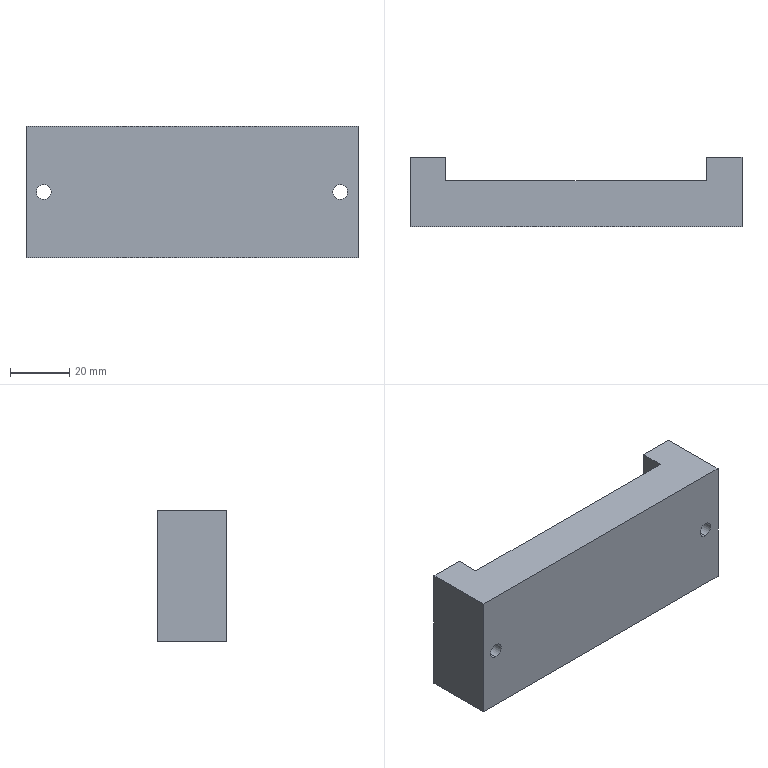Part | SolidWorks | features BaseBody 1 | 1 solid | 14 faces | box 112 x 23.5 x 44.5 mm | volume 84873 mm3 | plane 10 | cylinder 4 | commonest cylinder face diameters 5 x4
STEP:
#1=CARTESIAN_POINT('',(50.,-108.5,226.731));
#2=VERTEX_POINT('',#1);
#3=CARTESIAN_POINT('',(50.,-108.5,221.731));
#4=VERTEX_POINT('',#3);
#5=CARTESIAN_POINT('',(50.,-108.5,224.231));
#6=DIRECTION('',(0.,-1.,0.));
#7=DIRECTION('',(0.,0.,1.));
#8=AXIS2_PLACEMENT_3D('',#5,#6,#7);
#9=CIRCLE('',#8,2.5);
#10=EDGE_CURVE('',#2,#4,#9,.T.);
#11=ORIENTED_EDGE('',*,*,#10,.T.);
#12=CARTESIAN_POINT('',(50.,-85.,221.731));
#13=VERTEX_POINT('',#12);
#14=CARTESIAN_POINT('',(50.,-85.,221.731));
#15=DIRECTION('',(0.,1.,0.));
#16=VECTOR('',#15,1000.);
#17=LINE('',#14,#16);
#18=EDGE_CURVE('',#4,#13,#17,.T.);
#19=ORIENTED_EDGE('',*,*,#18,.T.);
#20=CARTESIAN_POINT('',(50.,-85.,226.731));
#21=VERTEX_POINT('',#20);
#22=CARTESIAN_POINT('',(50.,-85.,224.231));
#23=DIRECTION('',(0.,-1.,0.));
#24=DIRECTION('',(0.,0.,1.));
#25=AXIS2_PLACEMENT_3D('',#22,#23,#24);
#26=CIRCLE('',#25,2.5);
#27=EDGE_CURVE('',#21,#13,#26,.T.);
#28=ORIENTED_EDGE('',*,*,#27,.F.);
#29=CARTESIAN_POINT('',(50.,-85.,226.731));
#30=DIRECTION('',(0.,1.,0.));
#31=VECTOR('',#30,1000.);
#32=LINE('',#29,#31);
#33=EDGE_CURVE('',#2,#21,#32,.T.);
#34=ORIENTED_EDGE('',*,*,#33,.F.);
#35=EDGE_LOOP('',(#11,#19,#28,#34));
#36=FACE_OUTER_BOUND('',#35,.T.);
#37=CARTESIAN_POINT('',(50.,-85.,224.231));
#38=DIRECTION('',(0.,1.,0.));
#39=DIRECTION('',(0.,0.,1.));
#40=AXIS2_PLACEMENT_3D('',#37,#38,#39);
#41=CYLINDRICAL_SURFACE('',#40,2.5);
#42=ADVANCED_FACE('',(#36),#41,.F.);
#43=CARTESIAN_POINT('',(-50.,-108.5,226.731));
#44=VERTEX_POINT('',#43);
#45=CARTESIAN_POINT('',(-50.,-108.5,221.731));
#46=VERTEX_POINT('',#45);
#47=CARTESIAN_POINT('',(-50.,-108.5,224.231));
#48=DIRECTION('',(0.,-1.,0.));
#49=DIRECTION('',(0.,0.,1.));
#50=AXIS2_PLACEMENT_3D('',#47,#48,#49);
#51=CIRCLE('',#50,2.5);
#52=EDGE_CURVE('',#44,#46,#51,.T.);
#53=ORIENTED_EDGE('',*,*,#52,.T.);
#54=CARTESIAN_POINT('',(-50.,-85.,221.731));
#55=VERTEX_POINT('',#54);
#56=CARTESIAN_POINT('',(-50.,-85.,221.731));
#57=DIRECTION('',(0.,1.,0.));
#58=VECTOR('',#57,1000.);
#59=LINE('',#56,#58);
#60=EDGE_CURVE('',#46,#55,#59,.T.);
#61=ORIENTED_EDGE('',*,*,#60,.T.);
#62=CARTESIAN_POINT('',(-50.,-85.,226.731));
#63=VERTEX_POINT('',#62);
#64=CARTESIAN_POINT('',(-50.,-85.,224.231));
#65=DIRECTION('',(0.,-1.,0.));
#66=DIRECTION('',(0.,0.,1.));
#67=AXIS2_PLACEMENT_3D('',#64,#65,#66);
#68=CIRCLE('',#67,2.5);
#69=EDGE_CURVE('',#63,#55,#68,.T.);
#70=ORIENTED_EDGE('',*,*,#69,.F.);
#71=CARTESIAN_POINT('',(-50.,-85.,226.731));
#72=DIRECTION('',(0.,1.,0.));
#73=VECTOR('',#72,1000.);
#74=LINE('',#71,#73);
#75=EDGE_CURVE('',#44,#63,#74,.T.);
#76=ORIENTED_EDGE('',*,*,#75,.F.);
#77=EDGE_LOOP('',(#53,#61,#70,#76));
#78=FACE_OUTER_BOUND('',#77,.T.);
#79=CARTESIAN_POINT('',(-50.,-85.,224.231));
#80=DIRECTION('',(0.,1.,0.));
#81=DIRECTION('',(0.,0.,1.));
#82=AXIS2_PLACEMENT_3D('',#79,#80,#81);
#83=CYLINDRICAL_SURFACE('',#82,2.5);
#84=ADVANCED_FACE('',(#78),#83,.F.);
#85=CARTESIAN_POINT('',(56.,-108.5,246.481));
#86=VERTEX_POINT('',#85);
#87=CARTESIAN_POINT('',(56.,-108.5,201.981));
#88=VERTEX_POINT('',#87);
#89=CARTESIAN_POINT('',(56.,-108.5,246.481));
#90=DIRECTION('',(0.,0.,-1.));
#91=VECTOR('',#90,1000.);
#92=LINE('',#89,#91);
#93=EDGE_CURVE('',#86,#88,#92,.T.);
#94=ORIENTED_EDGE('',*,*,#93,.F.);
#95=CARTESIAN_POINT('',(-56.,-108.5,246.481));
#96=VERTEX_POINT('',#95);
#97=CARTESIAN_POINT('',(-56.,-108.5,246.481));
#98=DIRECTION('',(1.,0.,0.));
#99=VECTOR('',#98,1000.);
#100=LINE('',#97,#99);
#101=EDGE_CURVE('',#96,#86,#100,.T.);
#102=ORIENTED_EDGE('',*,*,#101,.F.);
#103=CARTESIAN_POINT('',(-56.,-108.5,201.981));
#104=VERTEX_POINT('',#103);
#105=CARTESIAN_POINT('',(-56.,-108.5,246.481));
#106=DIRECTION('',(0.,0.,1.));
#107=VECTOR('',#106,1000.);
#108=LINE('',#105,#107);
#109=EDGE_CURVE('',#104,#96,#108,.T.);
#110=ORIENTED_EDGE('',*,*,#109,.F.);
#111=CARTESIAN_POINT('',(-56.,-108.5,201.981));
#112=DIRECTION('',(-1.,0.,0.));
#113=VECTOR('',#112,1000.);
#114=LINE('',#111,#113);
#115=EDGE_CURVE('',#88,#104,#114,.T.);
#116=ORIENTED_EDGE('',*,*,#115,.F.);
#117=EDGE_LOOP('',(#94,#102,#110,#116));
#118=FACE_OUTER_BOUND('',#117,.T.);
#119=ORIENTED_EDGE('',*,*,#10,.F.);
#120=CARTESIAN_POINT('',(50.,-108.5,224.231));
#121=DIRECTION('',(0.,-1.,0.));
#122=DIRECTION('',(0.,0.,1.));
#123=AXIS2_PLACEMENT_3D('',#120,#121,#122);
#124=CIRCLE('',#123,2.5);
#125=EDGE_CURVE('',#4,#2,#124,.T.);
#126=ORIENTED_EDGE('',*,*,#125,.F.);
#127=EDGE_LOOP('',(#119,#126));
#128=FACE_BOUND('',#127,.T.);
#129=ORIENTED_EDGE('',*,*,#52,.F.);
#130=CARTESIAN_POINT('',(-50.,-108.5,224.231));
#131=DIRECTION('',(0.,-1.,0.));
#132=DIRECTION('',(0.,0.,1.));
#133=AXIS2_PLACEMENT_3D('',#130,#131,#132);
#134=CIRCLE('',#133,2.5);
#135=EDGE_CURVE('',#46,#44,#134,.T.);
#136=ORIENTED_EDGE('',*,*,#135,.F.);
#137=EDGE_LOOP('',(#129,#136));
#138=FACE_BOUND('',#137,.T.);
#139=CARTESIAN_POINT('',(-56.,-108.5,246.481));
#140=DIRECTION('',(0.,1.,0.));
#141=DIRECTION('',(0.,0.,1.));
#142=AXIS2_PLACEMENT_3D('',#139,#140,#141);
#143=PLANE('',#142);
#144=ADVANCED_FACE('',(#118,#128,#138),#143,.F.);
#145=ORIENTED_EDGE('',*,*,#115,.T.);
#146=CARTESIAN_POINT('',(-56.,-85.,201.981));
#147=VERTEX_POINT('',#146);
#148=CARTESIAN_POINT('',(-56.,-96.75,201.981));
#149=DIRECTION('',(0.,-1.,0.));
#150=VECTOR('',#149,1000.);
#151=LINE('',#148,#150);
#152=EDGE_CURVE('',#147,#104,#151,.T.);
#153=ORIENTED_EDGE('',*,*,#152,.F.);
#154=CARTESIAN_POINT('',(-44.,-85.,201.981));
#155=VERTEX_POINT('',#154);
#156=CARTESIAN_POINT('',(0.,-85.,201.981));
#157=DIRECTION('',(-1.,0.,0.));
#158=VECTOR('',#157,1000.);
#159=LINE('',#156,#158);
#160=EDGE_CURVE('',#155,#147,#159,.T.);
#161=ORIENTED_EDGE('',*,*,#160,.F.);
#162=CARTESIAN_POINT('',(-44.,-93.,201.981));
#163=VERTEX_POINT('',#162);
#164=CARTESIAN_POINT('',(-44.,-96.75,201.981));
#165=DIRECTION('',(0.,1.,0.));
#166=VECTOR('',#165,1000.);
#167=LINE('',#164,#166);
#168=EDGE_CURVE('',#163,#155,#167,.T.);
#169=ORIENTED_EDGE('',*,*,#168,.F.);
#170=CARTESIAN_POINT('',(44.,-93.,201.981));
#171=VERTEX_POINT('',#170);
#172=CARTESIAN_POINT('',(0.,-93.,201.981));
#173=DIRECTION('',(-1.,0.,0.));
#174=VECTOR('',#173,1000.);
#175=LINE('',#172,#174);
#176=EDGE_CURVE('',#171,#163,#175,.T.);
#177=ORIENTED_EDGE('',*,*,#176,.F.);
#178=CARTESIAN_POINT('',(44.,-85.,201.981));
#179=VERTEX_POINT('',#178);
#180=CARTESIAN_POINT('',(44.,-96.75,201.981));
#181=DIRECTION('',(0.,-1.,0.));
#182=VECTOR('',#181,1000.);
#183=LINE('',#180,#182);
#184=EDGE_CURVE('',#179,#171,#183,.T.);
#185=ORIENTED_EDGE('',*,*,#184,.F.);
#186=CARTESIAN_POINT('',(56.,-85.,201.981));
#187=VERTEX_POINT('',#186);
#188=CARTESIAN_POINT('',(0.,-85.,201.981));
#189=DIRECTION('',(-1.,0.,0.));
#190=VECTOR('',#189,1000.);
#191=LINE('',#188,#190);
#192=EDGE_CURVE('',#187,#179,#191,.T.);
#193=ORIENTED_EDGE('',*,*,#192,.F.);
#194=CARTESIAN_POINT('',(56.,-96.75,201.981));
#195=DIRECTION('',(0.,1.,0.));
#196=VECTOR('',#195,1000.);
#197=LINE('',#194,#196);
#198=EDGE_CURVE('',#88,#187,#197,.T.);
#199=ORIENTED_EDGE('',*,*,#198,.F.);
#200=EDGE_LOOP('',(#145,#153,#161,#169,#177,#185,#193,#199));
#201=FACE_OUTER_BOUND('',#200,.T.);
#202=CARTESIAN_POINT('',(0.,-96.75,201.981));
#203=DIRECTION('',(0.,0.,1.));
#204=DIRECTION('',(1.,0.,0.));
#205=AXIS2_PLACEMENT_3D('',#202,#203,#204);
#206=PLANE('',#205);
#207=ADVANCED_FACE('',(#201),#206,.F.);
#208=CARTESIAN_POINT('',(56.,-85.,246.481));
#209=VERTEX_POINT('',#208);
#210=CARTESIAN_POINT('',(56.,-85.,246.481));
#211=DIRECTION('',(0.,0.,-1.));
#212=VECTOR('',#211,1000.);
#213=LINE('',#210,#212);
#214=EDGE_CURVE('',#209,#187,#213,.T.);
#215=ORIENTED_EDGE('',*,*,#214,.F.);
#216=CARTESIAN_POINT('',(56.,-85.,246.481));
#217=DIRECTION('',(0.,1.,0.));
#218=VECTOR('',#217,1000.);
#219=LINE('',#216,#218);
#220=EDGE_CURVE('',#86,#209,#219,.T.);
#221=ORIENTED_EDGE('',*,*,#220,.F.);
#222=ORIENTED_EDGE('',*,*,#93,.T.);
#223=ORIENTED_EDGE('',*,*,#198,.T.);
#224=EDGE_LOOP('',(#215,#221,#222,#223));
#225=FACE_OUTER_BOUND('',#224,.T.);
#226=CARTESIAN_POINT('',(56.,-85.,246.481));
#227=DIRECTION('',(-1.,0.,0.));
#228=DIRECTION('',(0.,0.,1.));
#229=AXIS2_PLACEMENT_3D('',#226,#227,#228);
#230=PLANE('',#229);
#231=ADVANCED_FACE('',(#225),#230,.F.);
#232=CARTESIAN_POINT('',(-56.,-85.,246.481));
#233=VERTEX_POINT('',#232);
#234=CARTESIAN_POINT('',(-56.,-96.75,246.481));
#235=DIRECTION('',(0.,-1.,0.));
#236=VECTOR('',#235,1000.);
#237=LINE('',#234,#236);
#238=EDGE_CURVE('',#233,#96,#237,.T.);
#239=ORIENTED_EDGE('',*,*,#238,.T.);
#240=ORIENTED_EDGE('',*,*,#101,.T.);
#241=ORIENTED_EDGE('',*,*,#220,.T.);
#242=CARTESIAN_POINT('',(44.,-85.,246.481));
#243=VERTEX_POINT('',#242);
#244=CARTESIAN_POINT('',(0.,-85.,246.481));
#245=DIRECTION('',(-1.,0.,0.));
#246=VECTOR('',#245,1000.);
#247=LINE('',#244,#246);
#248=EDGE_CURVE('',#209,#243,#247,.T.);
#249=ORIENTED_EDGE('',*,*,#248,.T.);
#250=CARTESIAN_POINT('',(44.,-93.,246.481));
#251=VERTEX_POINT('',#250);
#252=CARTESIAN_POINT('',(44.,-96.75,246.481));
#253=DIRECTION('',(0.,-1.,0.));
#254=VECTOR('',#253,1000.);
#255=LINE('',#252,#254);
#256=EDGE_CURVE('',#243,#251,#255,.T.);
#257=ORIENTED_EDGE('',*,*,#256,.T.);
#258=CARTESIAN_POINT('',(-44.,-93.,246.481));
#259=VERTEX_POINT('',#258);
#260=CARTESIAN_POINT('',(0.,-93.,246.481));
#261=DIRECTION('',(-1.,0.,0.));
#262=VECTOR('',#261,1000.);
#263=LINE('',#260,#262);
#264=EDGE_CURVE('',#251,#259,#263,.T.);
#265=ORIENTED_EDGE('',*,*,#264,.T.);
#266=CARTESIAN_POINT('',(-44.,-85.,246.481));
#267=VERTEX_POINT('',#266);
#268=CARTESIAN_POINT('',(-44.,-96.75,246.481));
#269=DIRECTION('',(0.,1.,0.));
#270=VECTOR('',#269,1000.);
#271=LINE('',#268,#270);
#272=EDGE_CURVE('',#259,#267,#271,.T.);
#273=ORIENTED_EDGE('',*,*,#272,.T.);
#274=CARTESIAN_POINT('',(0.,-85.,246.481));
#275=DIRECTION('',(-1.,0.,0.));
#276=VECTOR('',#275,1000.);
#277=LINE('',#274,#276);
#278=EDGE_CURVE('',#267,#233,#277,.T.);
#279=ORIENTED_EDGE('',*,*,#278,.T.);
#280=EDGE_LOOP('',(#239,#240,#241,#249,#257,#265,#273,#279));
#281=FACE_OUTER_BOUND('',#280,.T.);
#282=CARTESIAN_POINT('',(0.,-96.75,246.481));
#283=DIRECTION('',(0.,0.,1.));
#284=DIRECTION('',(1.,0.,0.));
#285=AXIS2_PLACEMENT_3D('',#282,#283,#284);
#286=PLANE('',#285);
#287=ADVANCED_FACE('',(#281),#286,.T.);
#288=ORIENTED_EDGE('',*,*,#109,.T.);
#289=ORIENTED_EDGE('',*,*,#238,.F.);
#290=CARTESIAN_POINT('',(-56.,-85.,246.481));
#291=DIRECTION('',(0.,0.,1.));
#292=VECTOR('',#291,1000.);
#293=LINE('',#290,#292);
#294=EDGE_CURVE('',#147,#233,#293,.T.);
#295=ORIENTED_EDGE('',*,*,#294,.F.);
#296=ORIENTED_EDGE('',*,*,#152,.T.);
#297=EDGE_LOOP('',(#288,#289,#295,#296));
#298=FACE_OUTER_BOUND('',#297,.T.);
#299=CARTESIAN_POINT('',(-56.,-85.,246.481));
#300=DIRECTION('',(1.,0.,0.));
#301=DIRECTION('',(0.,0.,-1.));
#302=AXIS2_PLACEMENT_3D('',#299,#300,#301);
#303=PLANE('',#302);
#304=ADVANCED_FACE('',(#298),#303,.F.);
#305=ORIENTED_EDGE('',*,*,#18,.F.);
#306=ORIENTED_EDGE('',*,*,#125,.T.);
#307=ORIENTED_EDGE('',*,*,#33,.T.);
#308=CARTESIAN_POINT('',(50.,-85.,224.231));
#309=DIRECTION('',(0.,-1.,0.));
#310=DIRECTION('',(0.,0.,1.));
#311=AXIS2_PLACEMENT_3D('',#308,#309,#310);
#312=CIRCLE('',#311,2.5);
#313=EDGE_CURVE('',#13,#21,#312,.T.);
#314=ORIENTED_EDGE('',*,*,#313,.F.);
#315=EDGE_LOOP('',(#305,#306,#307,#314));
#316=FACE_OUTER_BOUND('',#315,.T.);
#317=CARTESIAN_POINT('',(50.,-85.,224.231));
#318=DIRECTION('',(0.,1.,0.));
#319=DIRECTION('',(0.,0.,1.));
#320=AXIS2_PLACEMENT_3D('',#317,#318,#319);
#321=CYLINDRICAL_SURFACE('',#320,2.5);
#322=ADVANCED_FACE('',(#316),#321,.F.);
#323=ORIENTED_EDGE('',*,*,#60,.F.);
#324=ORIENTED_EDGE('',*,*,#135,.T.);
#325=ORIENTED_EDGE('',*,*,#75,.T.);
#326=CARTESIAN_POINT('',(-50.,-85.,224.231));
#327=DIRECTION('',(0.,-1.,0.));
#328=DIRECTION('',(0.,0.,1.));
#329=AXIS2_PLACEMENT_3D('',#326,#327,#328);
#330=CIRCLE('',#329,2.5);
#331=EDGE_CURVE('',#55,#63,#330,.T.);
#332=ORIENTED_EDGE('',*,*,#331,.F.);
#333=EDGE_LOOP('',(#323,#324,#325,#332));
#334=FACE_OUTER_BOUND('',#333,.T.);
#335=CARTESIAN_POINT('',(-50.,-85.,224.231));
#336=DIRECTION('',(0.,1.,0.));
#337=DIRECTION('',(0.,0.,1.));
#338=AXIS2_PLACEMENT_3D('',#335,#336,#337);
#339=CYLINDRICAL_SURFACE('',#338,2.5);
#340=ADVANCED_FACE('',(#334),#339,.F.);
#341=ORIENTED_EDGE('',*,*,#294,.T.);
#342=ORIENTED_EDGE('',*,*,#278,.F.);
#343=CARTESIAN_POINT('',(-44.,-85.,246.481));
#344=DIRECTION('',(0.,0.,1.));
#345=VECTOR('',#344,1000.);
#346=LINE('',#343,#345);
#347=EDGE_CURVE('',#155,#267,#346,.T.);
#348=ORIENTED_EDGE('',*,*,#347,.F.);
#349=ORIENTED_EDGE('',*,*,#160,.T.);
#350=EDGE_LOOP('',(#341,#342,#348,#349));
#351=FACE_OUTER_BOUND('',#350,.T.);
#352=ORIENTED_EDGE('',*,*,#69,.T.);
#353=ORIENTED_EDGE('',*,*,#331,.T.);
#354=EDGE_LOOP('',(#352,#353));
#355=FACE_BOUND('',#354,.T.);
#356=CARTESIAN_POINT('',(-56.,-85.,246.481));
#357=DIRECTION('',(0.,-1.,0.));
#358=DIRECTION('',(0.,0.,-1.));
#359=AXIS2_PLACEMENT_3D('',#356,#357,#358);
#360=PLANE('',#359);
#361=ADVANCED_FACE('',(#351,#355),#360,.F.);
#362=ORIENTED_EDGE('',*,*,#347,.T.);
#363=ORIENTED_EDGE('',*,*,#272,.F.);
#364=CARTESIAN_POINT('',(-44.,-93.,246.481));
#365=DIRECTION('',(0.,0.,1.));
#366=VECTOR('',#365,1000.);
#367=LINE('',#364,#366);
#368=EDGE_CURVE('',#163,#259,#367,.T.);
#369=ORIENTED_EDGE('',*,*,#368,.F.);
#370=ORIENTED_EDGE('',*,*,#168,.T.);
#371=EDGE_LOOP('',(#362,#363,#369,#370));
#372=FACE_OUTER_BOUND('',#371,.T.);
#373=CARTESIAN_POINT('',(-44.,-85.,246.481));
#374=DIRECTION('',(-1.,0.,0.));
#375=DIRECTION('',(0.,0.,1.));
#376=AXIS2_PLACEMENT_3D('',#373,#374,#375);
#377=PLANE('',#376);
#378=ADVANCED_FACE('',(#372),#377,.F.);
#379=ORIENTED_EDGE('',*,*,#368,.T.);
#380=ORIENTED_EDGE('',*,*,#264,.F.);
#381=CARTESIAN_POINT('',(44.,-93.,246.481));
#382=DIRECTION('',(0.,0.,1.));
#383=VECTOR('',#382,1000.);
#384=LINE('',#381,#383);
#385=EDGE_CURVE('',#171,#251,#384,.T.);
#386=ORIENTED_EDGE('',*,*,#385,.F.);
#387=ORIENTED_EDGE('',*,*,#176,.T.);
#388=EDGE_LOOP('',(#379,#380,#386,#387));
#389=FACE_OUTER_BOUND('',#388,.T.);
#390=CARTESIAN_POINT('',(-44.,-93.,246.481));
#391=DIRECTION('',(0.,-1.,0.));
#392=DIRECTION('',(0.,0.,-1.));
#393=AXIS2_PLACEMENT_3D('',#390,#391,#392);
#394=PLANE('',#393);
#395=ADVANCED_FACE('',(#389),#394,.F.);
#396=ORIENTED_EDGE('',*,*,#385,.T.);
#397=ORIENTED_EDGE('',*,*,#256,.F.);
#398=CARTESIAN_POINT('',(44.,-85.,246.481));
#399=DIRECTION('',(0.,0.,1.));
#400=VECTOR('',#399,1000.);
#401=LINE('',#398,#400);
#402=EDGE_CURVE('',#179,#243,#401,.T.);
#403=ORIENTED_EDGE('',*,*,#402,.F.);
#404=ORIENTED_EDGE('',*,*,#184,.T.);
#405=EDGE_LOOP('',(#396,#397,#403,#404));
#406=FACE_OUTER_BOUND('',#405,.T.);
#407=CARTESIAN_POINT('',(44.,-93.,246.481));
#408=DIRECTION('',(1.,0.,0.));
#409=DIRECTION('',(0.,0.,-1.));
#410=AXIS2_PLACEMENT_3D('',#407,#408,#409);
#411=PLANE('',#410);
#412=ADVANCED_FACE('',(#406),#411,.F.);
#413=ORIENTED_EDGE('',*,*,#402,.T.);
#414=ORIENTED_EDGE('',*,*,#248,.F.);
#415=ORIENTED_EDGE('',*,*,#214,.T.);
#416=ORIENTED_EDGE('',*,*,#192,.T.);
#417=EDGE_LOOP('',(#413,#414,#415,#416));
#418=FACE_OUTER_BOUND('',#417,.T.);
#419=ORIENTED_EDGE('',*,*,#27,.T.);
#420=ORIENTED_EDGE('',*,*,#313,.T.);
#421=EDGE_LOOP('',(#419,#420));
#422=FACE_BOUND('',#421,.T.);
#423=CARTESIAN_POINT('',(44.,-85.,246.481));
#424=DIRECTION('',(0.,-1.,0.));
#425=DIRECTION('',(0.,0.,-1.));
#426=AXIS2_PLACEMENT_3D('',#423,#424,#425);
#427=PLANE('',#426);
#428=ADVANCED_FACE('',(#418,#422),#427,.F.);
#429=CLOSED_SHELL('',(#42,#84,#144,#207,#231,#287,#304,#322,#340,#361,#378,#395,#412,#428));
#430=MANIFOLD_SOLID_BREP('',#429);
#431=CARTESIAN_POINT('',(0.,0.,0.));
#432=DIRECTION('',(0.,0.,1.));
#433=DIRECTION('',(1.,0.,0.));
#434=AXIS2_PLACEMENT_3D('',#431,#432,#433);
#435=(LENGTH_UNIT()NAMED_UNIT(*)SI_UNIT(.MILLI.,.METRE.));
#436=UNCERTAINTY_MEASURE_WITH_UNIT(LENGTH_MEASURE(0.00001),#435,'','');
#437=(NAMED_UNIT(*)PLANE_ANGLE_UNIT()SI_UNIT($,.RADIAN.));
#438=(NAMED_UNIT(*)SI_UNIT($,.STERADIAN.)SOLID_ANGLE_UNIT());
#439=(GEOMETRIC_REPRESENTATION_CONTEXT(3)GLOBAL_UNCERTAINTY_ASSIGNED_CONTEXT((#436))GLOBAL_UNIT_ASSIGNED_CONTEXT((#435,#437,#438))REPRESENTATION_CONTEXT('',''));
#440=ADVANCED_BREP_SHAPE_REPRESENTATION('',(#430,#434),#439);